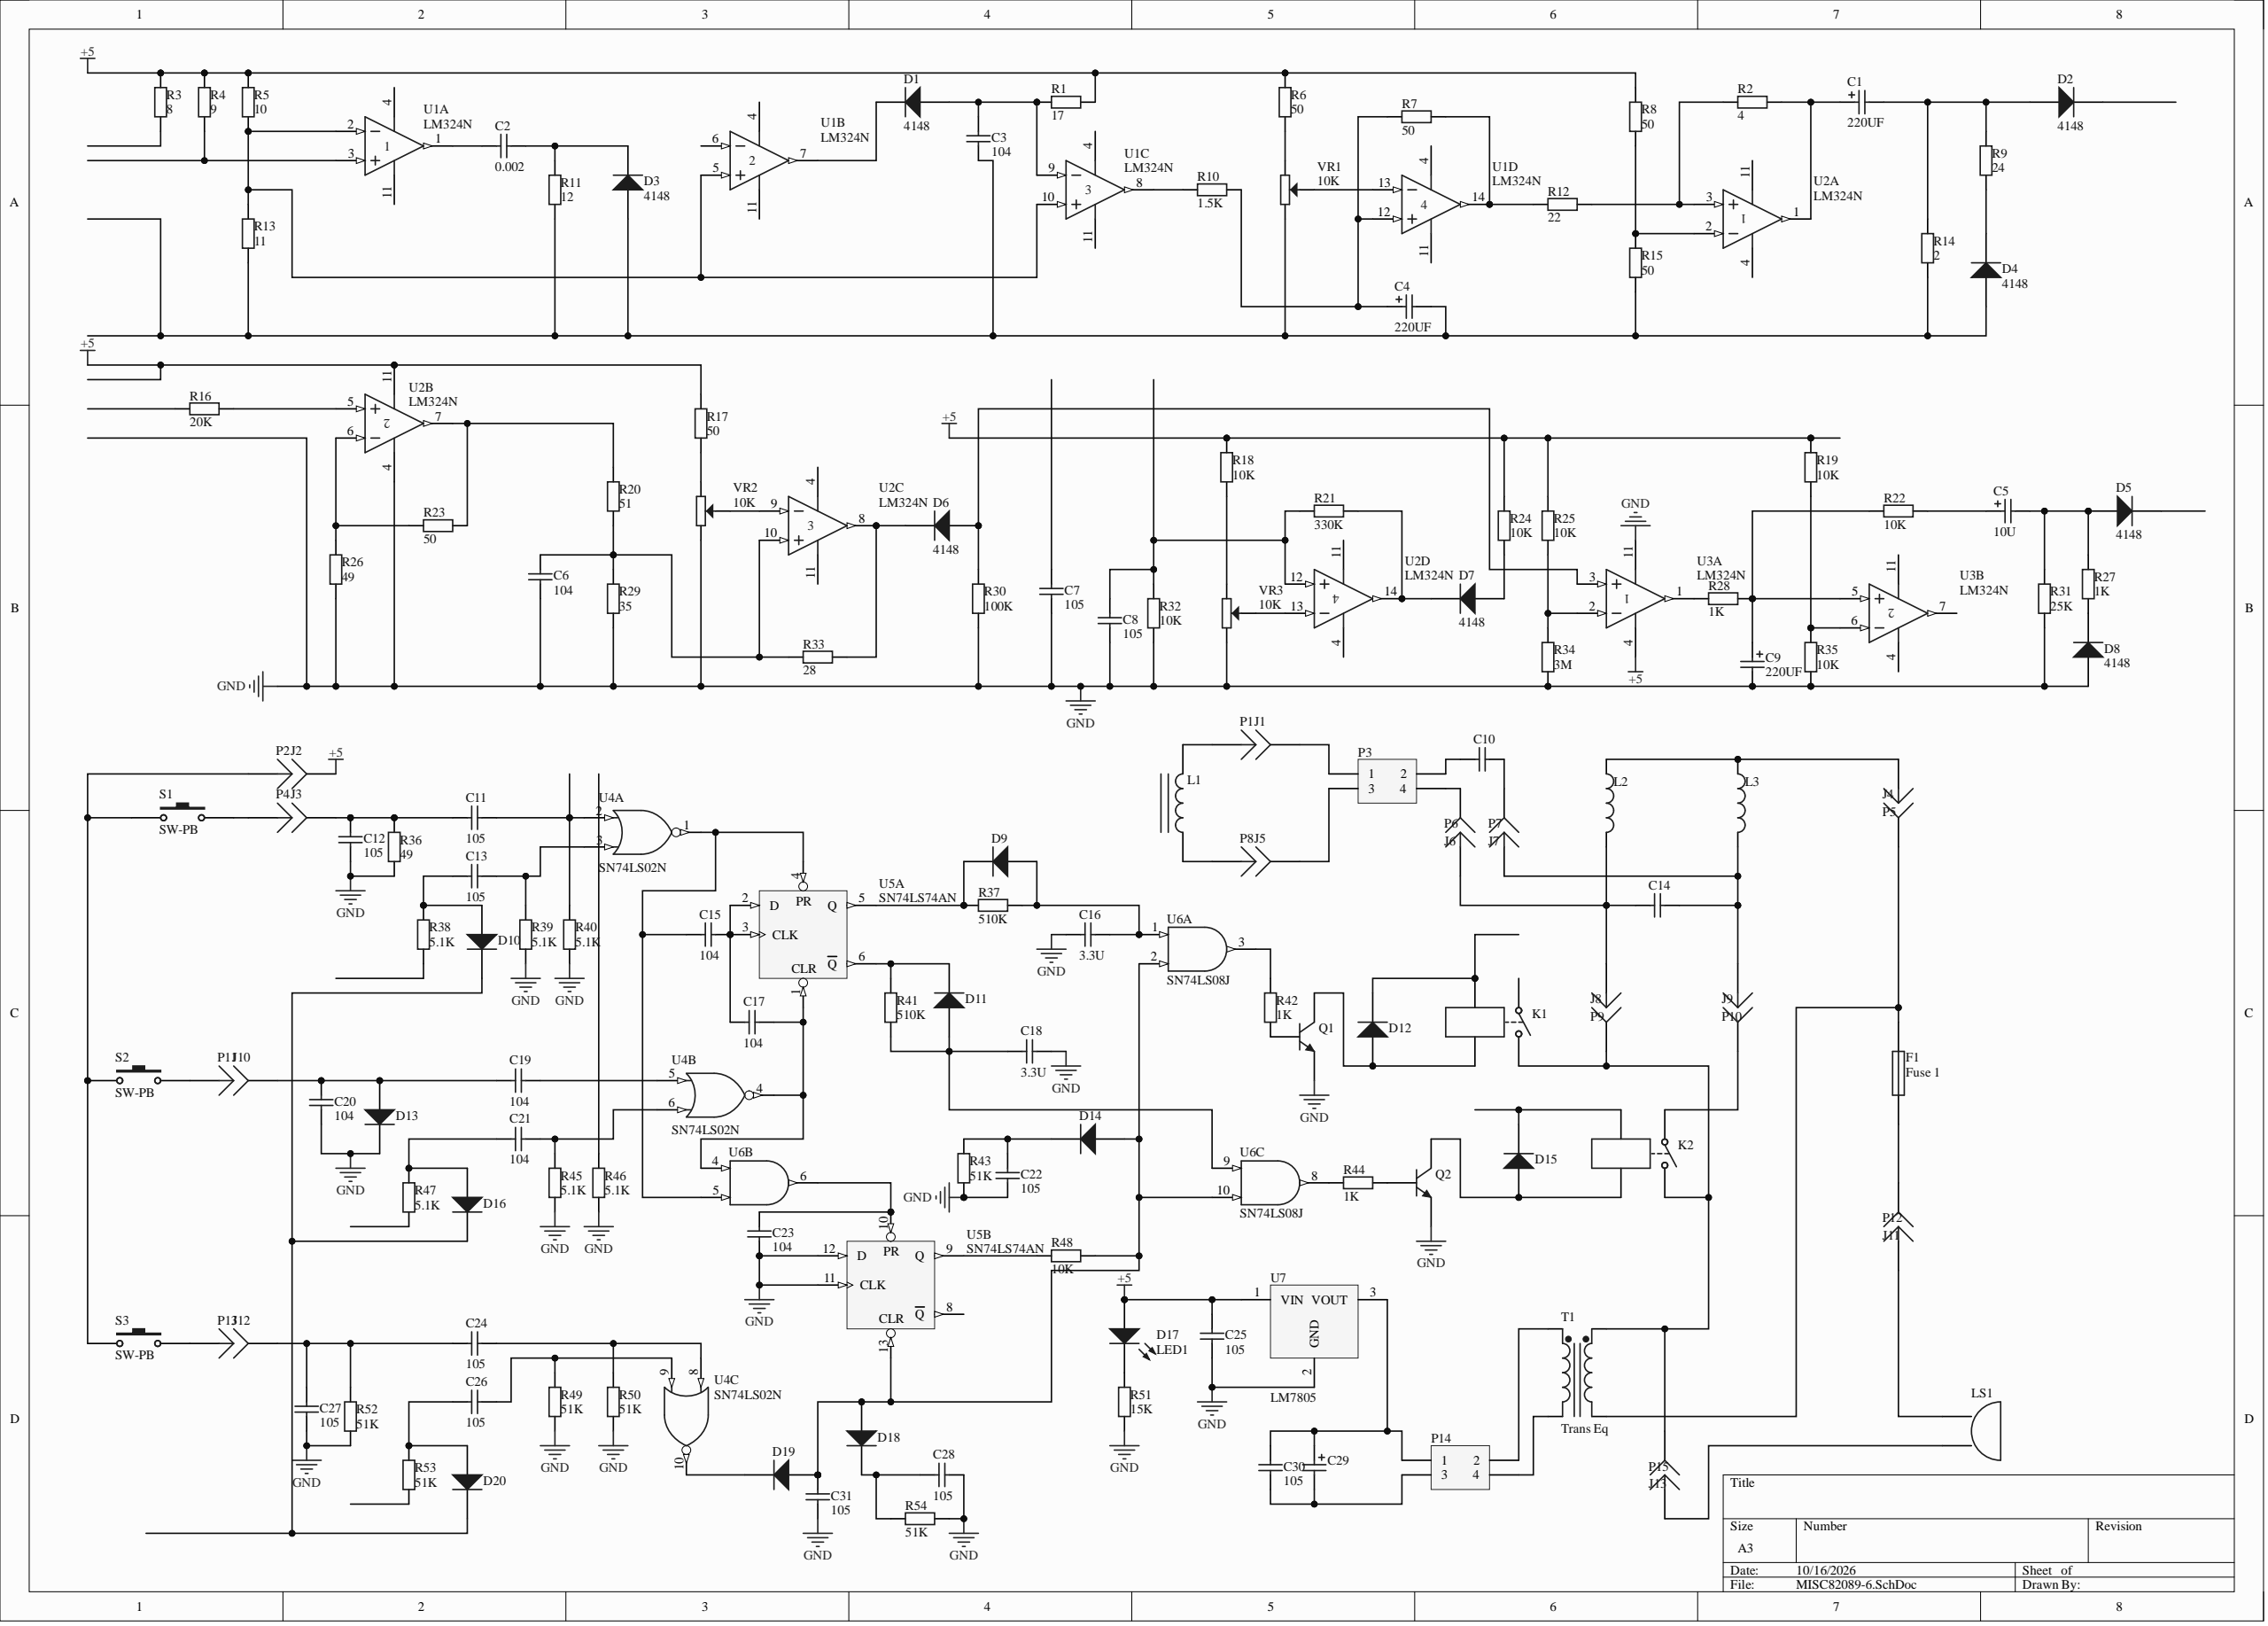Circuit board | Altium Designer | 156 parts | 99 nets
Bill of materials:
Comment,Description,Designator,Footprint,LibRef,Quantity
"220UF","Polarized Capacitor (Axial)","C1, C4, C9, C29","POLAR0.8","Cap Pol2","4"
"0.002","Capacitor","C2","RAD-0.2","Cap","1"
"104","Capacitor","C3, C6, C15, C17, C19, C20, C21, C23","RAD-0.2","Cap","8"
"10U","Polarized Capacitor (Axial)","C5","POLAR0.8","Cap Pol2","1"
"105","Capacitor","C7, C8, C11, C12, C13, C22, C24, C25, C26, C27, C28, C30, C31","RAD-0.2","Cap","13"
"3.3U","Capacitor","C10, C14, C16, C18","RAD-0.2","Cap","4"
"4148","High Conductance Fast Diode","D1, D2, D3, D4, D5, D6, D7, D8, D9, D10, D11, D12, D13, D14, D15, D16, D18, D19, D20","DO-35","Diode 1N914","19"
"LED1","Typical RED GaAs LED","D17","LED-1","LED1","1"
"Fuse 1","Fuse","F1","PIN-W2/E2.8","Fuse 1","1"
"Socket","Socket","J1, J2, J3, J4, J5, J6, J7, J8, J9, J10, J11, J12, J13","PIN1","Socket","13"
"Relay-SPST","Single-Pole Single-Throw Relay","K1, K2","MODULE4","Relay-SPST","2"
"Inductor Iron","Magnetic-Core Inductor","L1","AXIAL-0.9","Inductor Iron","1"
"Inductor","Inductor","L2, L3","0402-A","Inductor","2"
"Bell","Electrical Bell","LS1","PIN2","Bell","1"
"Plug","Plug","P1, P2, P4, P5, P6, P7, P8, P9, P10, P11, P12, P13, P15","PIN1","Plug","13"
"Header 2X2","Header, 2-Pin, Dual row","P3, P14","HDR2X2","Header 2X2","2"
"2N3904","NPN General Purpose Amplifier","Q1, Q2","TO-92A","2N3904","2"
"17","Resistor","R1","AXIAL-0.4","Res2","1"
"4","Resistor","R2","AXIAL-0.4","Res2","1"
"8","Resistor","R3","AXIAL-0.4","Res2","1"
"9","Resistor","R4","AXIAL-0.4","Res2","1"
"10","Resistor","R5","AXIAL-0.4","Res2","1"
"50","Resistor","R6, R7, R8, R15, R17, R23","AXIAL-0.4","Res2","6"
"24","Resistor","R9","AXIAL-0.4","Res2","1"
"1.5K","Resistor","R10","AXIAL-0.4","Res2","1"
"12","Resistor","R11","AXIAL-0.4","Res2","1"
"22","Resistor","R12","AXIAL-0.4","Res2","1"
"11","Resistor","R13","AXIAL-0.4","Res2","1"
"2","Resistor","R14","AXIAL-0.4","Res2","1"
"20K","Resistor","R16","AXIAL-0.4","Res2","1"
"10K","Resistor","R18, R19, R22, R24, R25, R32, R35, R48","AXIAL-0.4","Res2","8"
"51","Resistor","R20","AXIAL-0.4","Res2","1"
"330K","Resistor","R21","AXIAL-0.4","Res2","1"
"49","Resistor","R26, R36","AXIAL-0.4","Res2","2"
"1K","Resistor","R27, R28, R42, R44","AXIAL-0.4","Res2","4"
"35","Resistor","R29","AXIAL-0.4","Res2","1"
"100K","Resistor","R30","AXIAL-0.4","Res2","1"
"25K","Resistor","R31","AXIAL-0.4","Res2","1"
"28","Resistor","R33","AXIAL-0.4","Res2","1"
"3M","Resistor","R34","AXIAL-0.4","Res2","1"
"510K","Resistor","R37, R41","AXIAL-0.4","Res2","2"
"5.1K","Resistor","R38, R39, R40, R45, R46, R47","AXIAL-0.4","Res2","6"
"51K","Resistor","R43, R49, R50, R52, R53, R54","AXIAL-0.4","Res2","6"
"15K","Resistor","R51","AXIAL-0.4","Res2","1"
"SW-PB","Switch","S1, S2, S3","SPST-2","SW-PB","3"
"Trans Eq","Transformer (Equivalent Circuit Model)","T1","TRF_4","Trans Eq","1"
"LM324N","Quad Low-Power Operational Amplifier","U1, U2, U3","646-06","LM324N","3"
"SN74LS02N","Quadruple 2-Input Positive-NOR Gate","U4","N014","SN74LS02N","1"
"SN74LS74AN","Dual D-Type Positive Edge-Triggered Flip-Flop","U5","646-06","SN74LS74AN","1"
"SN74LS08J","Quadruple 2-Input Positive-AND Gate","U6","J014","SN74LS08J","1"
"LM7805","","U7","TO220A","LM7805","1"
"10K","","VR1, VR2, VR3","3296W","RESVR","3"
Netlist (Protel format):
[
C1
POLAR0.8
220UF



]
[
C2
RAD-0.2
0.002



]
[
C3
RAD-0.2
104



]
[
C4
POLAR0.8
220UF



]
[
C5
POLAR0.8
10U



]
[
C6
RAD-0.2
104



]
[
C7
RAD-0.2
105



]
[
C8
RAD-0.2
105



]
[
C9
POLAR0.8
220UF



]
[
C10
RAD-0.2
3.3U



]
[
C11
RAD-0.2
105



]
[
C12
RAD-0.2
105



]
[
C13
RAD-0.2
105



]
[
C14
RAD-0.2
3.3U



]
[
C15
RAD-0.2
104



]
[
C16
RAD-0.2
3.3U



]
[
C17
RAD-0.2
104



]
[
C18
RAD-0.2
3.3U



]
[
C19
RAD-0.2
104



]
[
C20
RAD-0.2
104



]
[
C21
RAD-0.2
104



]
[
C22
RAD-0.2
105



]
[
C23
RAD-0.2
104



]
[
C24
RAD-0.2
105



]
[
C25
RAD-0.2
105



]
[
C26
RAD-0.2
105



]
[
C27
RAD-0.2
105



]
[
C28
RAD-0.2
105



]
[
C29
POLAR0.8
220UF



]
[
C30
RAD-0.2
105



]
[
C31
RAD-0.2
105



]
[
D1
DO-35
4148



]
[
D2
DO-35
4148



]
[
D3
DO-35
4148



]
[
D4
DO-35
4148



]
[
D5
DO-35
4148



]
[
D6
DO-35
4148



]
[
D7
DO-35
4148



]
[
D8
DO-35
4148



]
[
D9
DO-35
4148



]
[
D10
DO-35
4148



]
[
D11
DO-35
4148



]
[
D12
DO-35
4148



]
[
D13
DO-35
4148



]
[
D14
DO-35
4148



]
[
D15
DO-35
4148



]
[
D16
DO-35
4148



]
[
D17
LED-1
LED1



]
[
D18
DO-35
4148



]
[
D19
DO-35
4148



]
[
D20
DO-35
4148



]
[
F1
PIN-W2/E2.8
Fuse 1



]
[
J1
PIN1
Socket



]
[
J2
PIN1
Socket



]
[
J3
PIN1
Socket



]
[
J4
PIN1
Socket



]
[
J5
PIN1
Socket



]
[
J6
PIN1
Socket



]
[
J7
PIN1
Socket



]
[
J8
PIN1
Socket



]
[
J9
PIN1
Socket



]
[
J10
PIN1
Socket



]
[
J11
PIN1
Socket



]
[
J12
PIN1
Socket



]
[
J13
PIN1
Socket



]
[
K1
MODULE4
Relay-SPST



]
[
K2
MODULE4
Relay-SPST



]
[
L1
AXIAL-0.9
Inductor Iron



]
[
L2
0402-A
Inductor



]
[
L3
0402-A
Inductor



]
[
LS1
PIN2
Bell



]
[
P1
PIN1
Plug



]
[
P2
PIN1
Plug



]
[
P3
HDR2X2
Header 2X2



]
[
P4
PIN1
Plug



]
[
P5
PIN1
Plug



]
[
P6
PIN1
Plug



]
[
P7
PIN1
Plug



]
[
P8
PIN1
Plug



]
[
P9
PIN1
Plug



]
[
P10
PIN1
Plug



]
[
P11
PIN1
Plug



]
[
P12
PIN1
Plug



]
[
P13
PIN1
Plug



]
[
P14
HDR2X2
Header 2X2



]
[
P15
PIN1
Plug



]
[
Q1
TO-92A
2N3904



]
[
Q2
TO-92A
2N3904



]
[
R1
AXIAL-0.4
17



]
[
R2
AXIAL-0.4
4



]
[
R3
AXIAL-0.4
8



]
[
R4
AXIAL-0.4
9



]
[
R5
AXIAL-0.4
10



]
[
R6
AXIAL-0.4
50



]
[
R7
AXIAL-0.4
50



]
[
R8
AXIAL-0.4
50



]
[
R9
AXIAL-0.4
24



]
[
R10
AXIAL-0.4
1.5K



]
[
R11
AXIAL-0.4
12



]
[
R12
AXIAL-0.4
22



]
[
R13
AXIAL-0.4
11



]
[
R14
AXIAL-0.4
2



]
[
R15
AXIAL-0.4
50



]
[
R16
AXIAL-0.4
20K



]
[
R17
AXIAL-0.4
50



]
[
R18
AXIAL-0.4
10K



]
[
R19
AXIAL-0.4
10K



]
[
R20
AXIAL-0.4
51



]
[
R21
AXIAL-0.4
330K



]
[
R22
AXIAL-0.4
10K



]
[
R23
AXIAL-0.4
50



]
[
R24
AXIAL-0.4
10K



]
[
R25
AXIAL-0.4
10K



]
[
R26
AXIAL-0.4
49



]
[
R27
AXIAL-0.4
1K



]
[
R28
AXIAL-0.4
1K



]
[
R29
AXIAL-0.4
35



]
[
R30
AXIAL-0.4
100K



]
[
R31
AXIAL-0.4
25K



]
[
R32
AXIAL-0.4
10K



]
[
R33
AXIAL-0.4
28



]
[
R34
AXIAL-0.4
3M



]
[
R35
AXIAL-0.4
10K



]
[
R36
AXIAL-0.4
49



]
[
R37
AXIAL-0.4
510K



]
[
R38
AXIAL-0.4
5.1K



]
[
R39
AXIAL-0.4
5.1K



]
[
R40
AXIAL-0.4
5.1K



]
[
R41
AXIAL-0.4
510K



]
[
R42
AXIAL-0.4
1K



]
[
R43
AXIAL-0.4
51K



]
[
R44
AXIAL-0.4
1K



]
[
R45
AXIAL-0.4
5.1K



]
[
R46
AXIAL-0.4
5.1K



]
[
R47
AXIAL-0.4
5.1K



]
[
R48
AXIAL-0.4
10K



]
[
R49
AXIAL-0.4
51K



]
[
R50
AXIAL-0.4
51K



]
[
R51
AXIAL-0.4
15K



]
[
R52
AXIAL-0.4
51K



]
[
R53
AXIAL-0.4
51K



]
[
R54
AXIAL-0.4
51K



]
[
S1
SPST-2
SW-PB



]
[
S2
SPST-2
SW-PB



]
[
S3
SPST-2
SW-PB



]
[
T1
TRF_4
Trans Eq



]
[
U1
646-06
LM324N



]
[
U2
646-06
LM324N



]
[
U3
646-06
LM324N



]
[
U4
N014
SN74LS02N



]
[
U5
646-06
SN74LS74AN



]
[
U6
J014
SN74LS08J



]
[
U7
TO220A
LM7805



]
[
VR1
3296W
10K



]
[
VR2
3296W
10K



]
[
VR3
3296W
10K



]
(
VCC
U4-14
U6-14
)
(
NetU2_13
U2-13
VR3-2
)
(
NetU2_9
U2-9
VR2-2
)
(
NetU1_13
U1-13
VR1-2
)
(
NetR48_1
R48-1
U5-9
)
(
NetR44_1
R44-1
U6-8
)
(
NetR42_1
R42-1
U6-3
)
(
NetR28_1
R28-1
U3-1
)
(
NetR25_2
R25-2
R34-1
U3-2
)
(
NetR23_2
R23-2
R26-1
U2-6
)
(
NetR20_1
R20-1
R23-1
U2-7
)
(
NetR19_2
R19-2
R35-1
U3-6
)
(
NetR18_2
R18-2
VR3-1
)
(
NetR17_2
R17-2
VR2-1
)
(
NetR16_1
R16-1
U2-5
)
(
NetR10_1
R10-1
U1-8
)
(
NetR8_1
R8-1
R15-2
U2-2
)
(
NetR7_2
R7-2
R12-1
U1-14
)
(
NetR6_2
R6-2
VR1-1
)
(
NetR5_1
R5-1
R13-2
U1-2
U1-5
U1-10
)
(
NetR4_1
R4-1
U1-3
)
(
NetR2_2
R2-2
R12-2
U2-3
)
(
NetQ2_2
Q2-2
R44-2
)
(
NetQ1_2
Q1-2
R42-2
)
(
NetP14_4
P14-4
T1-2
)
(
NetP14_2
P14-2
T1-1
)
(
NetP13_1
P13-1
S3-2
)
(
NetP11_1
P11-1
S2-2
)
(
NetP4_1
P4-1
S1-2
)
(
NetP2_1
P2-1
S1-1
S2-1
S3-1
)
(
NetLS1_2
LS1-2
P15-1
)
(
NetLS1_1
LS1-1
P12-1
)
(
NetL2_1
L2-1
L3-1
P5-1
)
(
NetL1_2
L1-2
P1-1
)
(
NetL1_1
L1-1
P8-1
)
(
NetJ9_1
J9-1
K2-1
)
(
NetJ8_1
J8-1
J13-1
K1-2
K2-2
T1-3
)
(
NetJ6_1
J6-1
P3-4
)
(
NetJ5_1
J5-1
P3-3
)
(
NetJ1_1
J1-1
P3-1
)
(
NetF1_2
F1-2
J4-1
T1-4
)
(
NetF1_1
F1-1
J11-1
)
(
NetD19_2
D19-2
U4-10
)
(
NetD17_2
D17-2
R51-2
)
(
NetD15_2
D15-2
K2-3
)
(
NetD15_1
D15-1
K2-4
Q2-3
)
(
NetD12_2
D12-2
K1-3
)
(
NetD12_1
D12-1
K1-4
Q1-3
)
(
NetD11_2
D11-2
R41-1
U5-6
)
(
NetD10_2
D10-2
D16-2
D20-2
)
(
NetD9_2
D9-2
R37-1
U5-5
)
(
NetD8_2
D8-2
R27-1
)
(
NetD7_2
D7-2
R21-2
U2-14
)
(
NetD7_1
D7-1
R24-2
)
(
NetD6_2
D6-2
R33-2
U2-8
)
(
NetD6_1
D6-1
R30-2
U3-3
)
(
NetD4_2
D4-2
R9-2
)
(
NetD1_2
D1-2
U1-7
)
(
NetC31_1
C31-1
D14-1
D18-1
D19-1
R48-2
U5-13
U6-2
U6-10
)
(
NetC29_2
C29-2
C30-1
P14-3
)
(
NetC29_1
C29-1
C30-2
P14-1
U7-3
)
(
NetC28_2
C28-2
D18-2
R54-1
)
(
NetC26_2
C26-2
D20-1
R53-1
)
(
NetC26_1
C26-1
R49-1
U4-9
)
(
NetC24_2
C24-2
C27-1
J12-1
R52-1
)
(
NetC24_1
C24-1
R50-1
U4-8
)
(
NetC23_2
C23-2
U5-10
U6-6
)
(
NetC22_2
C22-2
D14-2
R43-1
)
(
NetC21_2
C21-2
R45-1
U4-6
)
(
NetC21_1
C21-1
D16-1
R47-1
)
(
NetC19_2
C19-2
U4-5
)
(
NetC19_1
C19-1
C20-2
D13-1
J10-1
)
(
NetC18_1
C18-1
D11-1
R41-2
U6-9
)
(
NetC17_2
C17-2
U4-4
U5-1
U6-4
)
(
NetC16_2
C16-2
D9-1
R37-2
U6-1
)
(
NetC15_2
C15-2
C17-1
U5-2
U5-3
)
(
NetC15_1
C15-1
U4-1
U5-4
U6-5
)
(
NetC14_2
C14-2
L3-2
P7-1
P10-1
)
(
NetC14_1
C14-1
L2-2
P6-1
P9-1
)
(
NetC13_2
C13-2
R39-1
U4-3
)
(
NetC13_1
C13-1
D10-1
R38-1
)
(
NetC11_2
C11-2
R40-1
U4-2
)
(
NetC11_1
C11-1
C12-2
J3-1
R36-1
)
(
NetC10_2
C10-2
J7-1
)
(
NetC10_1
C10-1
P3-2
)
(
NetC9_1
C9-1
R22-1
R28-2
U3-5
)
(
NetC8_1
C8-1
R21-1
R32-2
U2-12
)
(
NetC6_2
C6-2
R20-2
R29-1
R33-1
U2-10
)
(
NetC5_2
C5-2
D5-1
R27-2
R31-1
)
(
NetC5_1
C5-1
R22-2
)
(
NetC4_1
C4-1
R7-1
R10-2
U1-12
)
(
NetC3_2
C3-2
D1-1
R1-1
U1-9
)
(
NetC3_1
C3-1
C4-2
D3-1
D4-1
R11-1
R13-1
R14-2
R15-1
VR1-2
)
(
NetC2_2
C2-2
D3-2
R11-2
)
(
NetC2_1
C2-1
U1-1
)
(
NetC1_2
C1-2
D2-1
R9-1
R14-1
)
(
NetC1_1
C1-1
R2-1
U2-1
)
(
GND
C6-1
C7-2
C8-2
C9-2
C12-1
C16-1
C18-2
C20-1
C22-1
C23-1
C25-1
C27-2
C28-1
C31-2
D8-1
D13-2
Q1-1
Q2-1
R26-2
R29-2
R30-1
R31-2
R32-1
R34-2
R35-2
R36-2
R39-2
R40-2
R43-2
R45-2
R46-2
R49-2
R50-2
R51-1
R52-2
R54-2
U2-4
U3-11
U4-7
U5-7
U5-11
U5-12
U6-7
U7-2
VR2-2
VR3-2
)
(
+5
C25-2
D17-1
J2-1
R1-2
R3-2
R4-2
R5-2
R6-1
R8-2
R17-1
R18-1
R19-1
R24-1
R25-1
U2-11
U3-4
U7-1
)